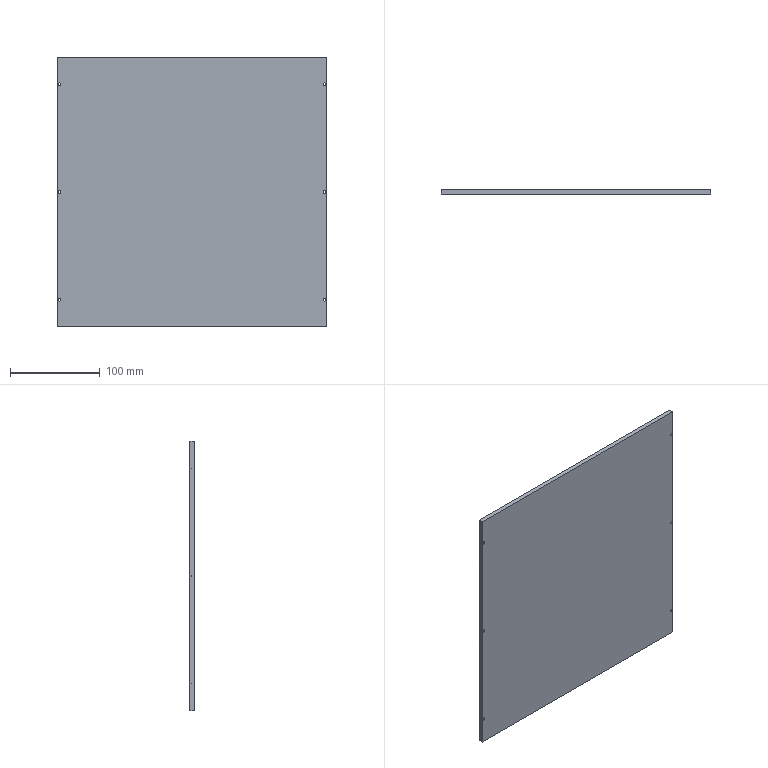Part | SolidWorks | features Extrusion 1, HoleWzd 1 | 1 solid | 30 faces | box 300 x 5 x 300 mm | volume 449761 mm3 | cylinder 12 | cone 12 | plane 6 | commonest cylinder face diameters 2.7 x12
STEP:
#1=CARTESIAN_POINT('',(147.5,0.,-118.65));
#2=VERTEX_POINT('',#1);
#3=CARTESIAN_POINT('',(147.5,0.,-121.35));
#4=VERTEX_POINT('',#3);
#5=CARTESIAN_POINT('',(147.5,0.,-120.));
#6=DIRECTION('',(0.,-1.,0.));
#7=DIRECTION('',(0.,0.,-1.));
#8=AXIS2_PLACEMENT_3D('',#5,#6,#7);
#9=CIRCLE('',#8,1.35);
#10=EDGE_CURVE('',#2,#4,#9,.T.);
#11=ORIENTED_EDGE('',*,*,#10,.T.);
#12=CARTESIAN_POINT('',(147.5,3.6,-121.35));
#13=VERTEX_POINT('',#12);
#14=CARTESIAN_POINT('',(147.5,5.,-121.35));
#15=DIRECTION('',(0.,1.,0.));
#16=VECTOR('',#15,1000.);
#17=LINE('',#14,#16);
#18=EDGE_CURVE('',#4,#13,#17,.T.);
#19=ORIENTED_EDGE('',*,*,#18,.T.);
#20=CARTESIAN_POINT('',(147.5,3.6,-118.65));
#21=VERTEX_POINT('',#20);
#22=CARTESIAN_POINT('',(147.5,3.6,-120.));
#23=DIRECTION('',(0.,1.,0.));
#24=DIRECTION('',(0.,0.,1.));
#25=AXIS2_PLACEMENT_3D('',#22,#23,#24);
#26=CIRCLE('',#25,1.35);
#27=EDGE_CURVE('',#13,#21,#26,.T.);
#28=ORIENTED_EDGE('',*,*,#27,.T.);
#29=CARTESIAN_POINT('',(147.5,5.,-118.65));
#30=DIRECTION('',(0.,1.,0.));
#31=VECTOR('',#30,1000.);
#32=LINE('',#29,#31);
#33=EDGE_CURVE('',#2,#21,#32,.T.);
#34=ORIENTED_EDGE('',*,*,#33,.F.);
#35=EDGE_LOOP('',(#11,#19,#28,#34));
#36=FACE_OUTER_BOUND('',#35,.T.);
#37=CARTESIAN_POINT('',(147.5,5.,-120.));
#38=DIRECTION('',(0.,1.,0.));
#39=DIRECTION('',(0.,0.,1.));
#40=AXIS2_PLACEMENT_3D('',#37,#38,#39);
#41=CYLINDRICAL_SURFACE('',#40,1.35);
#42=ADVANCED_FACE('',(#36),#41,.F.);
#43=ORIENTED_EDGE('',*,*,#27,.F.);
#44=CARTESIAN_POINT('',(147.5,5.,-122.75));
#45=VERTEX_POINT('',#44);
#46=CARTESIAN_POINT('',(147.5,5.,-122.75));
#47=DIRECTION('',(0.,0.7071,-0.7071));
#48=VECTOR('',#47,1000.);
#49=LINE('',#46,#48);
#50=EDGE_CURVE('',#13,#45,#49,.T.);
#51=ORIENTED_EDGE('',*,*,#50,.T.);
#52=CARTESIAN_POINT('',(147.5,5.,-117.25));
#53=VERTEX_POINT('',#52);
#54=CARTESIAN_POINT('',(147.5,5.,-120.));
#55=DIRECTION('',(0.,1.,0.));
#56=DIRECTION('',(0.,0.,1.));
#57=AXIS2_PLACEMENT_3D('',#54,#55,#56);
#58=CIRCLE('',#57,2.75);
#59=EDGE_CURVE('',#45,#53,#58,.T.);
#60=ORIENTED_EDGE('',*,*,#59,.T.);
#61=CARTESIAN_POINT('',(147.5,5.,-117.25));
#62=DIRECTION('',(0.,0.7071,0.7071));
#63=VECTOR('',#62,1000.);
#64=LINE('',#61,#63);
#65=EDGE_CURVE('',#21,#53,#64,.T.);
#66=ORIENTED_EDGE('',*,*,#65,.F.);
#67=EDGE_LOOP('',(#43,#51,#60,#66));
#68=FACE_OUTER_BOUND('',#67,.T.);
#69=CARTESIAN_POINT('',(147.5,5.,-120.));
#70=DIRECTION('',(0.,1.,0.));
#71=DIRECTION('',(0.,0.,1.));
#72=AXIS2_PLACEMENT_3D('',#69,#70,#71);
#73=CONICAL_SURFACE('',#72,2.75,0.7854);
#74=ADVANCED_FACE('',(#68),#73,.F.);
#75=CARTESIAN_POINT('',(147.5,0.,1.35));
#76=VERTEX_POINT('',#75);
#77=CARTESIAN_POINT('',(147.5,0.,-1.35));
#78=VERTEX_POINT('',#77);
#79=CARTESIAN_POINT('',(147.5,0.,0.));
#80=DIRECTION('',(0.,-1.,0.));
#81=DIRECTION('',(0.,0.,-1.));
#82=AXIS2_PLACEMENT_3D('',#79,#80,#81);
#83=CIRCLE('',#82,1.35);
#84=EDGE_CURVE('',#76,#78,#83,.T.);
#85=ORIENTED_EDGE('',*,*,#84,.T.);
#86=CARTESIAN_POINT('',(147.5,3.6,-1.35));
#87=VERTEX_POINT('',#86);
#88=CARTESIAN_POINT('',(147.5,5.,-1.35));
#89=DIRECTION('',(0.,1.,0.));
#90=VECTOR('',#89,1000.);
#91=LINE('',#88,#90);
#92=EDGE_CURVE('',#78,#87,#91,.T.);
#93=ORIENTED_EDGE('',*,*,#92,.T.);
#94=CARTESIAN_POINT('',(147.5,3.6,1.35));
#95=VERTEX_POINT('',#94);
#96=CARTESIAN_POINT('',(147.5,3.6,0.));
#97=DIRECTION('',(0.,1.,0.));
#98=DIRECTION('',(0.,0.,1.));
#99=AXIS2_PLACEMENT_3D('',#96,#97,#98);
#100=CIRCLE('',#99,1.35);
#101=EDGE_CURVE('',#87,#95,#100,.T.);
#102=ORIENTED_EDGE('',*,*,#101,.T.);
#103=CARTESIAN_POINT('',(147.5,5.,1.35));
#104=DIRECTION('',(0.,1.,0.));
#105=VECTOR('',#104,1000.);
#106=LINE('',#103,#105);
#107=EDGE_CURVE('',#76,#95,#106,.T.);
#108=ORIENTED_EDGE('',*,*,#107,.F.);
#109=EDGE_LOOP('',(#85,#93,#102,#108));
#110=FACE_OUTER_BOUND('',#109,.T.);
#111=CARTESIAN_POINT('',(147.5,5.,0.));
#112=DIRECTION('',(0.,1.,0.));
#113=DIRECTION('',(0.,0.,1.));
#114=AXIS2_PLACEMENT_3D('',#111,#112,#113);
#115=CYLINDRICAL_SURFACE('',#114,1.35);
#116=ADVANCED_FACE('',(#110),#115,.F.);
#117=ORIENTED_EDGE('',*,*,#101,.F.);
#118=CARTESIAN_POINT('',(147.5,5.,-2.75));
#119=VERTEX_POINT('',#118);
#120=CARTESIAN_POINT('',(147.5,5.,-2.75));
#121=DIRECTION('',(0.,0.7071,-0.7071));
#122=VECTOR('',#121,1000.);
#123=LINE('',#120,#122);
#124=EDGE_CURVE('',#87,#119,#123,.T.);
#125=ORIENTED_EDGE('',*,*,#124,.T.);
#126=CARTESIAN_POINT('',(147.5,5.,2.75));
#127=VERTEX_POINT('',#126);
#128=CARTESIAN_POINT('',(147.5,5.,0.));
#129=DIRECTION('',(0.,1.,0.));
#130=DIRECTION('',(0.,0.,1.));
#131=AXIS2_PLACEMENT_3D('',#128,#129,#130);
#132=CIRCLE('',#131,2.75);
#133=EDGE_CURVE('',#119,#127,#132,.T.);
#134=ORIENTED_EDGE('',*,*,#133,.T.);
#135=CARTESIAN_POINT('',(147.5,5.,2.75));
#136=DIRECTION('',(0.,0.7071,0.7071));
#137=VECTOR('',#136,1000.);
#138=LINE('',#135,#137);
#139=EDGE_CURVE('',#95,#127,#138,.T.);
#140=ORIENTED_EDGE('',*,*,#139,.F.);
#141=EDGE_LOOP('',(#117,#125,#134,#140));
#142=FACE_OUTER_BOUND('',#141,.T.);
#143=CARTESIAN_POINT('',(147.5,5.,0.));
#144=DIRECTION('',(0.,1.,0.));
#145=DIRECTION('',(0.,0.,1.));
#146=AXIS2_PLACEMENT_3D('',#143,#144,#145);
#147=CONICAL_SURFACE('',#146,2.75,0.7854);
#148=ADVANCED_FACE('',(#142),#147,.F.);
#149=CARTESIAN_POINT('',(147.5,0.,121.35));
#150=VERTEX_POINT('',#149);
#151=CARTESIAN_POINT('',(147.5,0.,118.65));
#152=VERTEX_POINT('',#151);
#153=CARTESIAN_POINT('',(147.5,0.,120.));
#154=DIRECTION('',(0.,-1.,0.));
#155=DIRECTION('',(0.,0.,-1.));
#156=AXIS2_PLACEMENT_3D('',#153,#154,#155);
#157=CIRCLE('',#156,1.35);
#158=EDGE_CURVE('',#150,#152,#157,.T.);
#159=ORIENTED_EDGE('',*,*,#158,.T.);
#160=CARTESIAN_POINT('',(147.5,3.6,118.65));
#161=VERTEX_POINT('',#160);
#162=CARTESIAN_POINT('',(147.5,5.,118.65));
#163=DIRECTION('',(0.,1.,0.));
#164=VECTOR('',#163,1000.);
#165=LINE('',#162,#164);
#166=EDGE_CURVE('',#152,#161,#165,.T.);
#167=ORIENTED_EDGE('',*,*,#166,.T.);
#168=CARTESIAN_POINT('',(147.5,3.6,121.35));
#169=VERTEX_POINT('',#168);
#170=CARTESIAN_POINT('',(147.5,3.6,120.));
#171=DIRECTION('',(0.,1.,0.));
#172=DIRECTION('',(0.,0.,1.));
#173=AXIS2_PLACEMENT_3D('',#170,#171,#172);
#174=CIRCLE('',#173,1.35);
#175=EDGE_CURVE('',#161,#169,#174,.T.);
#176=ORIENTED_EDGE('',*,*,#175,.T.);
#177=CARTESIAN_POINT('',(147.5,5.,121.35));
#178=DIRECTION('',(0.,1.,0.));
#179=VECTOR('',#178,1000.);
#180=LINE('',#177,#179);
#181=EDGE_CURVE('',#150,#169,#180,.T.);
#182=ORIENTED_EDGE('',*,*,#181,.F.);
#183=EDGE_LOOP('',(#159,#167,#176,#182));
#184=FACE_OUTER_BOUND('',#183,.T.);
#185=CARTESIAN_POINT('',(147.5,5.,120.));
#186=DIRECTION('',(0.,1.,0.));
#187=DIRECTION('',(0.,0.,1.));
#188=AXIS2_PLACEMENT_3D('',#185,#186,#187);
#189=CYLINDRICAL_SURFACE('',#188,1.35);
#190=ADVANCED_FACE('',(#184),#189,.F.);
#191=ORIENTED_EDGE('',*,*,#175,.F.);
#192=CARTESIAN_POINT('',(147.5,5.,117.25));
#193=VERTEX_POINT('',#192);
#194=CARTESIAN_POINT('',(147.5,5.,117.25));
#195=DIRECTION('',(0.,0.7071,-0.7071));
#196=VECTOR('',#195,1000.);
#197=LINE('',#194,#196);
#198=EDGE_CURVE('',#161,#193,#197,.T.);
#199=ORIENTED_EDGE('',*,*,#198,.T.);
#200=CARTESIAN_POINT('',(147.5,5.,122.75));
#201=VERTEX_POINT('',#200);
#202=CARTESIAN_POINT('',(147.5,5.,120.));
#203=DIRECTION('',(0.,1.,0.));
#204=DIRECTION('',(0.,0.,1.));
#205=AXIS2_PLACEMENT_3D('',#202,#203,#204);
#206=CIRCLE('',#205,2.75);
#207=EDGE_CURVE('',#193,#201,#206,.T.);
#208=ORIENTED_EDGE('',*,*,#207,.T.);
#209=CARTESIAN_POINT('',(147.5,5.,122.75));
#210=DIRECTION('',(0.,0.7071,0.7071));
#211=VECTOR('',#210,1000.);
#212=LINE('',#209,#211);
#213=EDGE_CURVE('',#169,#201,#212,.T.);
#214=ORIENTED_EDGE('',*,*,#213,.F.);
#215=EDGE_LOOP('',(#191,#199,#208,#214));
#216=FACE_OUTER_BOUND('',#215,.T.);
#217=CARTESIAN_POINT('',(147.5,5.,120.));
#218=DIRECTION('',(0.,1.,0.));
#219=DIRECTION('',(0.,0.,1.));
#220=AXIS2_PLACEMENT_3D('',#217,#218,#219);
#221=CONICAL_SURFACE('',#220,2.75,0.7854);
#222=ADVANCED_FACE('',(#216),#221,.F.);
#223=CARTESIAN_POINT('',(-147.5,0.,-118.65));
#224=VERTEX_POINT('',#223);
#225=CARTESIAN_POINT('',(-147.5,0.,-121.35));
#226=VERTEX_POINT('',#225);
#227=CARTESIAN_POINT('',(-147.5,0.,-120.));
#228=DIRECTION('',(0.,-1.,0.));
#229=DIRECTION('',(0.,0.,-1.));
#230=AXIS2_PLACEMENT_3D('',#227,#228,#229);
#231=CIRCLE('',#230,1.35);
#232=EDGE_CURVE('',#224,#226,#231,.T.);
#233=ORIENTED_EDGE('',*,*,#232,.T.);
#234=CARTESIAN_POINT('',(-147.5,3.6,-121.35));
#235=VERTEX_POINT('',#234);
#236=CARTESIAN_POINT('',(-147.5,5.,-121.35));
#237=DIRECTION('',(0.,1.,0.));
#238=VECTOR('',#237,1000.);
#239=LINE('',#236,#238);
#240=EDGE_CURVE('',#226,#235,#239,.T.);
#241=ORIENTED_EDGE('',*,*,#240,.T.);
#242=CARTESIAN_POINT('',(-147.5,3.6,-118.65));
#243=VERTEX_POINT('',#242);
#244=CARTESIAN_POINT('',(-147.5,3.6,-120.));
#245=DIRECTION('',(0.,1.,0.));
#246=DIRECTION('',(0.,0.,1.));
#247=AXIS2_PLACEMENT_3D('',#244,#245,#246);
#248=CIRCLE('',#247,1.35);
#249=EDGE_CURVE('',#235,#243,#248,.T.);
#250=ORIENTED_EDGE('',*,*,#249,.T.);
#251=CARTESIAN_POINT('',(-147.5,5.,-118.65));
#252=DIRECTION('',(0.,1.,0.));
#253=VECTOR('',#252,1000.);
#254=LINE('',#251,#253);
#255=EDGE_CURVE('',#224,#243,#254,.T.);
#256=ORIENTED_EDGE('',*,*,#255,.F.);
#257=EDGE_LOOP('',(#233,#241,#250,#256));
#258=FACE_OUTER_BOUND('',#257,.T.);
#259=CARTESIAN_POINT('',(-147.5,5.,-120.));
#260=DIRECTION('',(0.,1.,0.));
#261=DIRECTION('',(0.,0.,1.));
#262=AXIS2_PLACEMENT_3D('',#259,#260,#261);
#263=CYLINDRICAL_SURFACE('',#262,1.35);
#264=ADVANCED_FACE('',(#258),#263,.F.);
#265=ORIENTED_EDGE('',*,*,#249,.F.);
#266=CARTESIAN_POINT('',(-147.5,5.,-122.75));
#267=VERTEX_POINT('',#266);
#268=CARTESIAN_POINT('',(-147.5,5.,-122.75));
#269=DIRECTION('',(0.,0.7071,-0.7071));
#270=VECTOR('',#269,1000.);
#271=LINE('',#268,#270);
#272=EDGE_CURVE('',#235,#267,#271,.T.);
#273=ORIENTED_EDGE('',*,*,#272,.T.);
#274=CARTESIAN_POINT('',(-150.,5.,-121.146));
#275=VERTEX_POINT('',#274);
#276=CARTESIAN_POINT('',(-147.5,5.,-120.));
#277=DIRECTION('',(0.,1.,0.));
#278=DIRECTION('',(0.,0.,1.));
#279=AXIS2_PLACEMENT_3D('',#276,#277,#278);
#280=CIRCLE('',#279,2.75);
#281=EDGE_CURVE('',#267,#275,#280,.T.);
#282=ORIENTED_EDGE('',*,*,#281,.T.);
#283=CARTESIAN_POINT('',(-150.,5.,-118.854));
#284=VERTEX_POINT('',#283);
#285=CARTESIAN_POINT('',(-150.,5.,-118.854));
#286=CARTESIAN_POINT('',(-150.,4.924,-119.036));
#287=CARTESIAN_POINT('',(-150.,4.861,-119.225));
#288=CARTESIAN_POINT('',(-150.,4.774,-119.607));
#289=CARTESIAN_POINT('',(-150.,4.75,-119.802));
#290=CARTESIAN_POINT('',(-150.,4.75,-120.199));
#291=CARTESIAN_POINT('',(-150.,4.774,-120.394));
#292=CARTESIAN_POINT('',(-150.,4.861,-120.775));
#293=CARTESIAN_POINT('',(-150.,4.925,-120.965));
#294=CARTESIAN_POINT('',(-150.,5.,-121.146));
#295=B_SPLINE_CURVE_WITH_KNOTS('',3,(#285,#286,#287,#288,#289,#290,#291,#292,#293,#294),.UNSPECIFIED.,.F.,.F.,(4,2,2,2,4),(0.0116,0.01218,0.01277,0.01335,0.01394),.UNSPECIFIED.);
#296=EDGE_CURVE('',#284,#275,#295,.T.);
#297=ORIENTED_EDGE('',*,*,#296,.F.);
#298=CARTESIAN_POINT('',(-147.5,5.,-117.25));
#299=VERTEX_POINT('',#298);
#300=CARTESIAN_POINT('',(-147.5,5.,-120.));
#301=DIRECTION('',(0.,1.,0.));
#302=DIRECTION('',(0.,0.,1.));
#303=AXIS2_PLACEMENT_3D('',#300,#301,#302);
#304=CIRCLE('',#303,2.75);
#305=EDGE_CURVE('',#284,#299,#304,.T.);
#306=ORIENTED_EDGE('',*,*,#305,.T.);
#307=CARTESIAN_POINT('',(-147.5,5.,-117.25));
#308=DIRECTION('',(0.,0.7071,0.7071));
#309=VECTOR('',#308,1000.);
#310=LINE('',#307,#309);
#311=EDGE_CURVE('',#243,#299,#310,.T.);
#312=ORIENTED_EDGE('',*,*,#311,.F.);
#313=EDGE_LOOP('',(#265,#273,#282,#297,#306,#312));
#314=FACE_OUTER_BOUND('',#313,.T.);
#315=CARTESIAN_POINT('',(-147.5,5.,-120.));
#316=DIRECTION('',(0.,1.,0.));
#317=DIRECTION('',(0.,0.,1.));
#318=AXIS2_PLACEMENT_3D('',#315,#316,#317);
#319=CONICAL_SURFACE('',#318,2.75,0.7854);
#320=ADVANCED_FACE('',(#314),#319,.F.);
#321=CARTESIAN_POINT('',(-147.5,0.,1.35));
#322=VERTEX_POINT('',#321);
#323=CARTESIAN_POINT('',(-147.5,0.,-1.35));
#324=VERTEX_POINT('',#323);
#325=CARTESIAN_POINT('',(-147.5,0.,0.));
#326=DIRECTION('',(0.,-1.,0.));
#327=DIRECTION('',(0.,0.,-1.));
#328=AXIS2_PLACEMENT_3D('',#325,#326,#327);
#329=CIRCLE('',#328,1.35);
#330=EDGE_CURVE('',#322,#324,#329,.T.);
#331=ORIENTED_EDGE('',*,*,#330,.T.);
#332=CARTESIAN_POINT('',(-147.5,3.6,-1.35));
#333=VERTEX_POINT('',#332);
#334=CARTESIAN_POINT('',(-147.5,5.,-1.35));
#335=DIRECTION('',(0.,1.,0.));
#336=VECTOR('',#335,1000.);
#337=LINE('',#334,#336);
#338=EDGE_CURVE('',#324,#333,#337,.T.);
#339=ORIENTED_EDGE('',*,*,#338,.T.);
#340=CARTESIAN_POINT('',(-147.5,3.6,1.35));
#341=VERTEX_POINT('',#340);
#342=CARTESIAN_POINT('',(-147.5,3.6,0.));
#343=DIRECTION('',(0.,1.,0.));
#344=DIRECTION('',(0.,0.,1.));
#345=AXIS2_PLACEMENT_3D('',#342,#343,#344);
#346=CIRCLE('',#345,1.35);
#347=EDGE_CURVE('',#333,#341,#346,.T.);
#348=ORIENTED_EDGE('',*,*,#347,.T.);
#349=CARTESIAN_POINT('',(-147.5,5.,1.35));
#350=DIRECTION('',(0.,1.,0.));
#351=VECTOR('',#350,1000.);
#352=LINE('',#349,#351);
#353=EDGE_CURVE('',#322,#341,#352,.T.);
#354=ORIENTED_EDGE('',*,*,#353,.F.);
#355=EDGE_LOOP('',(#331,#339,#348,#354));
#356=FACE_OUTER_BOUND('',#355,.T.);
#357=CARTESIAN_POINT('',(-147.5,5.,0.));
#358=DIRECTION('',(0.,1.,0.));
#359=DIRECTION('',(0.,0.,1.));
#360=AXIS2_PLACEMENT_3D('',#357,#358,#359);
#361=CYLINDRICAL_SURFACE('',#360,1.35);
#362=ADVANCED_FACE('',(#356),#361,.F.);
#363=ORIENTED_EDGE('',*,*,#347,.F.);
#364=CARTESIAN_POINT('',(-147.5,5.,-2.75));
#365=VERTEX_POINT('',#364);
#366=CARTESIAN_POINT('',(-147.5,5.,-2.75));
#367=DIRECTION('',(0.,0.7071,-0.7071));
#368=VECTOR('',#367,1000.);
#369=LINE('',#366,#368);
#370=EDGE_CURVE('',#333,#365,#369,.T.);
#371=ORIENTED_EDGE('',*,*,#370,.T.);
#372=CARTESIAN_POINT('',(-150.,5.,-1.146));
#373=VERTEX_POINT('',#372);
#374=CARTESIAN_POINT('',(-147.5,5.,0.));
#375=DIRECTION('',(0.,1.,0.));
#376=DIRECTION('',(0.,0.,1.));
#377=AXIS2_PLACEMENT_3D('',#374,#375,#376);
#378=CIRCLE('',#377,2.75);
#379=EDGE_CURVE('',#365,#373,#378,.T.);
#380=ORIENTED_EDGE('',*,*,#379,.T.);
#381=CARTESIAN_POINT('',(-150.,5.,1.146));
#382=VERTEX_POINT('',#381);
#383=CARTESIAN_POINT('',(-150.,5.,1.146));
#384=CARTESIAN_POINT('',(-150.,4.924,0.9642));
#385=CARTESIAN_POINT('',(-150.,4.861,0.7753));
#386=CARTESIAN_POINT('',(-150.,4.774,0.3932));
#387=CARTESIAN_POINT('',(-150.,4.75,0.1976));
#388=CARTESIAN_POINT('',(-150.,4.75,-0.1993));
#389=CARTESIAN_POINT('',(-150.,4.774,-0.3936));
#390=CARTESIAN_POINT('',(-150.,4.861,-0.7755));
#391=CARTESIAN_POINT('',(-150.,4.925,-0.9646));
#392=CARTESIAN_POINT('',(-150.,5.,-1.146));
#393=B_SPLINE_CURVE_WITH_KNOTS('',3,(#383,#384,#385,#386,#387,#388,#389,#390,#391,#392),.UNSPECIFIED.,.F.,.F.,(4,2,2,2,4),(0.0116,0.01218,0.01277,0.01335,0.01394),.UNSPECIFIED.);
#394=EDGE_CURVE('',#382,#373,#393,.T.);
#395=ORIENTED_EDGE('',*,*,#394,.F.);
#396=CARTESIAN_POINT('',(-147.5,5.,2.75));
#397=VERTEX_POINT('',#396);
#398=CARTESIAN_POINT('',(-147.5,5.,0.));
#399=DIRECTION('',(0.,1.,0.));
#400=DIRECTION('',(0.,0.,1.));
#401=AXIS2_PLACEMENT_3D('',#398,#399,#400);
#402=CIRCLE('',#401,2.75);
#403=EDGE_CURVE('',#382,#397,#402,.T.);
#404=ORIENTED_EDGE('',*,*,#403,.T.);
#405=CARTESIAN_POINT('',(-147.5,5.,2.75));
#406=DIRECTION('',(0.,0.7071,0.7071));
#407=VECTOR('',#406,1000.);
#408=LINE('',#405,#407);
#409=EDGE_CURVE('',#341,#397,#408,.T.);
#410=ORIENTED_EDGE('',*,*,#409,.F.);
#411=EDGE_LOOP('',(#363,#371,#380,#395,#404,#410));
#412=FACE_OUTER_BOUND('',#411,.T.);
#413=CARTESIAN_POINT('',(-147.5,5.,0.));
#414=DIRECTION('',(0.,1.,0.));
#415=DIRECTION('',(0.,0.,1.));
#416=AXIS2_PLACEMENT_3D('',#413,#414,#415);
#417=CONICAL_SURFACE('',#416,2.75,0.7854);
#418=ADVANCED_FACE('',(#412),#417,.F.);
#419=CARTESIAN_POINT('',(-147.5,0.,121.35));
#420=VERTEX_POINT('',#419);
#421=CARTESIAN_POINT('',(-147.5,0.,118.65));
#422=VERTEX_POINT('',#421);
#423=CARTESIAN_POINT('',(-147.5,0.,120.));
#424=DIRECTION('',(0.,-1.,0.));
#425=DIRECTION('',(0.,0.,-1.));
#426=AXIS2_PLACEMENT_3D('',#423,#424,#425);
#427=CIRCLE('',#426,1.35);
#428=EDGE_CURVE('',#420,#422,#427,.T.);
#429=ORIENTED_EDGE('',*,*,#428,.T.);
#430=CARTESIAN_POINT('',(-147.5,3.6,118.65));
#431=VERTEX_POINT('',#430);
#432=CARTESIAN_POINT('',(-147.5,5.,118.65));
#433=DIRECTION('',(0.,1.,0.));
#434=VECTOR('',#433,1000.);
#435=LINE('',#432,#434);
#436=EDGE_CURVE('',#422,#431,#435,.T.);
#437=ORIENTED_EDGE('',*,*,#436,.T.);
#438=CARTESIAN_POINT('',(-147.5,3.6,121.35));
#439=VERTEX_POINT('',#438);
#440=CARTESIAN_POINT('',(-147.5,3.6,120.));
#441=DIRECTION('',(0.,1.,0.));
#442=DIRECTION('',(0.,0.,1.));
#443=AXIS2_PLACEMENT_3D('',#440,#441,#442);
#444=CIRCLE('',#443,1.35);
#445=EDGE_CURVE('',#431,#439,#444,.T.);
#446=ORIENTED_EDGE('',*,*,#445,.T.);
#447=CARTESIAN_POINT('',(-147.5,5.,121.35));
#448=DIRECTION('',(0.,1.,0.));
#449=VECTOR('',#448,1000.);
#450=LINE('',#447,#449);
#451=EDGE_CURVE('',#420,#439,#450,.T.);
#452=ORIENTED_EDGE('',*,*,#451,.F.);
#453=EDGE_LOOP('',(#429,#437,#446,#452));
#454=FACE_OUTER_BOUND('',#453,.T.);
#455=CARTESIAN_POINT('',(-147.5,5.,120.));
#456=DIRECTION('',(0.,1.,0.));
#457=DIRECTION('',(0.,0.,1.));
#458=AXIS2_PLACEMENT_3D('',#455,#456,#457);
#459=CYLINDRICAL_SURFACE('',#458,1.35);
#460=ADVANCED_FACE('',(#454),#459,.F.);
#461=ORIENTED_EDGE('',*,*,#445,.F.);
#462=CARTESIAN_POINT('',(-147.5,5.,117.25));
#463=VERTEX_POINT('',#462);
#464=CARTESIAN_POINT('',(-147.5,5.,117.25));
#465=DIRECTION('',(0.,0.7071,-0.7071));
#466=VECTOR('',#465,1000.);
#467=LINE('',#464,#466);
#468=EDGE_CURVE('',#431,#463,#467,.T.);
#469=ORIENTED_EDGE('',*,*,#468,.T.);
#470=CARTESIAN_POINT('',(-150.,5.,118.854));
#471=VERTEX_POINT('',#470);
#472=CARTESIAN_POINT('',(-147.5,5.,120.));
#473=DIRECTION('',(0.,1.,0.));
#474=DIRECTION('',(0.,0.,1.));
#475=AXIS2_PLACEMENT_3D('',#472,#473,#474);
#476=CIRCLE('',#475,2.75);
#477=EDGE_CURVE('',#463,#471,#476,.T.);
#478=ORIENTED_EDGE('',*,*,#477,.T.);
#479=CARTESIAN_POINT('',(-150.,5.,121.146));
#480=VERTEX_POINT('',#479);
#481=CARTESIAN_POINT('',(-150.,5.,121.146));
#482=CARTESIAN_POINT('',(-150.,4.924,120.964));
#483=CARTESIAN_POINT('',(-150.,4.861,120.775));
#484=CARTESIAN_POINT('',(-150.,4.774,120.393));
#485=CARTESIAN_POINT('',(-150.,4.75,120.198));
#486=CARTESIAN_POINT('',(-150.,4.75,119.801));
#487=CARTESIAN_POINT('',(-150.,4.774,119.606));
#488=CARTESIAN_POINT('',(-150.,4.861,119.225));
#489=CARTESIAN_POINT('',(-150.,4.925,119.035));
#490=CARTESIAN_POINT('',(-150.,5.,118.854));
#491=B_SPLINE_CURVE_WITH_KNOTS('',3,(#481,#482,#483,#484,#485,#486,#487,#488,#489,#490),.UNSPECIFIED.,.F.,.F.,(4,2,2,2,4),(0.0116,0.01218,0.01277,0.01335,0.01394),.UNSPECIFIED.);
#492=EDGE_CURVE('',#480,#471,#491,.T.);
#493=ORIENTED_EDGE('',*,*,#492,.F.);
#494=CARTESIAN_POINT('',(-147.5,5.,122.75));
#495=VERTEX_POINT('',#494);
#496=CARTESIAN_POINT('',(-147.5,5.,120.));
#497=DIRECTION('',(0.,1.,0.));
#498=DIRECTION('',(0.,0.,1.));
#499=AXIS2_PLACEMENT_3D('',#496,#497,#498);
#500=CIRCLE('',#499,2.75);
#501=EDGE_CURVE('',#480,#495,#500,.T.);
#502=ORIENTED_EDGE('',*,*,#501,.T.);
#503=CARTESIAN_POINT('',(-147.5,5.,122.75));
#504=DIRECTION('',(0.,0.7071,0.7071));
#505=VECTOR('',#504,1000.);
#506=LINE('',#503,#505);
#507=EDGE_CURVE('',#439,#495,#506,.T.);
#508=ORIENTED_EDGE('',*,*,#507,.F.);
#509=EDGE_LOOP('',(#461,#469,#478,#493,#502,#508));
#510=FACE_OUTER_BOUND('',#509,.T.);
#511=CARTESIAN_POINT('',(-147.5,5.,120.));
#512=DIRECTION('',(0.,1.,0.));
#513=DIRECTION('',(0.,0.,1.));
#514=AXIS2_PLACEMENT_3D('',#511,#512,#513);
#515=CONICAL_SURFACE('',#514,2.75,0.7854);
#516=ADVANCED_FACE('',(#510),#515,.F.);
#517=CARTESIAN_POINT('',(150.,5.,-1.146));
#518=VERTEX_POINT('',#517);
#519=CARTESIAN_POINT('',(150.,5.,-118.854));
#520=VERTEX_POINT('',#519);
#521=CARTESIAN_POINT('',(150.,5.,150.));
#522=DIRECTION('',(0.,0.,-1.));
#523=VECTOR('',#522,1000.);
#524=LINE('',#521,#523);
#525=EDGE_CURVE('',#518,#520,#524,.T.);
#526=ORIENTED_EDGE('',*,*,#525,.T.);
#527=CARTESIAN_POINT('',(147.5,5.,-120.));
#528=DIRECTION('',(0.,1.,0.));
#529=DIRECTION('',(0.,0.,1.));
#530=AXIS2_PLACEMENT_3D('',#527,#528,#529);
#531=CIRCLE('',#530,2.75);
#532=EDGE_CURVE('',#53,#520,#531,.T.);
#533=ORIENTED_EDGE('',*,*,#532,.F.);
#534=ORIENTED_EDGE('',*,*,#59,.F.);
#535=CARTESIAN_POINT('',(150.,5.,-121.146));
#536=VERTEX_POINT('',#535);
#537=CARTESIAN_POINT('',(147.5,5.,-120.));
#538=DIRECTION('',(0.,1.,0.));
#539=DIRECTION('',(0.,0.,1.));
#540=AXIS2_PLACEMENT_3D('',#537,#538,#539);
#541=CIRCLE('',#540,2.75);
#542=EDGE_CURVE('',#536,#45,#541,.T.);
#543=ORIENTED_EDGE('',*,*,#542,.F.);
#544=CARTESIAN_POINT('',(150.,5.,-150.));
#545=VERTEX_POINT('',#544);
#546=CARTESIAN_POINT('',(150.,5.,150.));
#547=DIRECTION('',(0.,0.,-1.));
#548=VECTOR('',#547,1000.);
#549=LINE('',#546,#548);
#550=EDGE_CURVE('',#536,#545,#549,.T.);
#551=ORIENTED_EDGE('',*,*,#550,.T.);
#552=CARTESIAN_POINT('',(-150.,5.,-150.));
#553=VERTEX_POINT('',#552);
#554=CARTESIAN_POINT('',(-150.,5.,-150.));
#555=DIRECTION('',(-1.,0.,0.));
#556=VECTOR('',#555,1000.);
#557=LINE('',#554,#556);
#558=EDGE_CURVE('',#545,#553,#557,.T.);
#559=ORIENTED_EDGE('',*,*,#558,.T.);
#560=CARTESIAN_POINT('',(-150.,5.,150.));
#561=DIRECTION('',(0.,0.,1.));
#562=VECTOR('',#561,1000.);
#563=LINE('',#560,#562);
#564=EDGE_CURVE('',#553,#275,#563,.T.);
#565=ORIENTED_EDGE('',*,*,#564,.T.);
#566=ORIENTED_EDGE('',*,*,#281,.F.);
#567=CARTESIAN_POINT('',(-147.5,5.,-120.));
#568=DIRECTION('',(0.,1.,0.));
#569=DIRECTION('',(0.,0.,1.));
#570=AXIS2_PLACEMENT_3D('',#567,#568,#569);
#571=CIRCLE('',#570,2.75);
#572=EDGE_CURVE('',#299,#267,#571,.T.);
#573=ORIENTED_EDGE('',*,*,#572,.F.);
#574=ORIENTED_EDGE('',*,*,#305,.F.);
#575=CARTESIAN_POINT('',(-150.,5.,150.));
#576=DIRECTION('',(0.,0.,1.));
#577=VECTOR('',#576,1000.);
#578=LINE('',#575,#577);
#579=EDGE_CURVE('',#284,#373,#578,.T.);
#580=ORIENTED_EDGE('',*,*,#579,.T.);
#581=ORIENTED_EDGE('',*,*,#379,.F.);
#582=CARTESIAN_POINT('',(-147.5,5.,0.));
#583=DIRECTION('',(0.,1.,0.));
#584=DIRECTION('',(0.,0.,1.));
#585=AXIS2_PLACEMENT_3D('',#582,#583,#584);
#586=CIRCLE('',#585,2.75);
#587=EDGE_CURVE('',#397,#365,#586,.T.);
#588=ORIENTED_EDGE('',*,*,#587,.F.);
#589=ORIENTED_EDGE('',*,*,#403,.F.);
#590=CARTESIAN_POINT('',(-150.,5.,150.));
#591=DIRECTION('',(0.,0.,1.));
#592=VECTOR('',#591,1000.);
#593=LINE('',#590,#592);
#594=EDGE_CURVE('',#382,#471,#593,.T.);
#595=ORIENTED_EDGE('',*,*,#594,.T.);
#596=ORIENTED_EDGE('',*,*,#477,.F.);
#597=CARTESIAN_POINT('',(-147.5,5.,120.));
#598=DIRECTION('',(0.,1.,0.));
#599=DIRECTION('',(0.,0.,1.));
#600=AXIS2_PLACEMENT_3D('',#597,#598,#599);
#601=CIRCLE('',#600,2.75);
#602=EDGE_CURVE('',#495,#463,#601,.T.);
#603=ORIENTED_EDGE('',*,*,#602,.F.);
#604=ORIENTED_EDGE('',*,*,#501,.F.);
#605=CARTESIAN_POINT('',(-150.,5.,150.));
#606=VERTEX_POINT('',#605);
#607=CARTESIAN_POINT('',(-150.,5.,150.));
#608=DIRECTION('',(0.,0.,1.));
#609=VECTOR('',#608,1000.);
#610=LINE('',#607,#609);
#611=EDGE_CURVE('',#480,#606,#610,.T.);
#612=ORIENTED_EDGE('',*,*,#611,.T.);
#613=CARTESIAN_POINT('',(150.,5.,150.));
#614=VERTEX_POINT('',#613);
#615=CARTESIAN_POINT('',(-150.,5.,150.));
#616=DIRECTION('',(1.,0.,0.));
#617=VECTOR('',#616,1000.);
#618=LINE('',#615,#617);
#619=EDGE_CURVE('',#606,#614,#618,.T.);
#620=ORIENTED_EDGE('',*,*,#619,.T.);
#621=CARTESIAN_POINT('',(150.,5.,121.146));
#622=VERTEX_POINT('',#621);
#623=CARTESIAN_POINT('',(150.,5.,150.));
#624=DIRECTION('',(0.,0.,-1.));
#625=VECTOR('',#624,1000.);
#626=LINE('',#623,#625);
#627=EDGE_CURVE('',#614,#622,#626,.T.);
#628=ORIENTED_EDGE('',*,*,#627,.T.);
#629=CARTESIAN_POINT('',(147.5,5.,120.));
#630=DIRECTION('',(0.,1.,0.));
#631=DIRECTION('',(0.,0.,1.));
#632=AXIS2_PLACEMENT_3D('',#629,#630,#631);
#633=CIRCLE('',#632,2.75);
#634=EDGE_CURVE('',#201,#622,#633,.T.);
#635=ORIENTED_EDGE('',*,*,#634,.F.);
#636=ORIENTED_EDGE('',*,*,#207,.F.);
#637=CARTESIAN_POINT('',(150.,5.,118.854));
#638=VERTEX_POINT('',#637);
#639=CARTESIAN_POINT('',(147.5,5.,120.));
#640=DIRECTION('',(0.,1.,0.));
#641=DIRECTION('',(0.,0.,1.));
#642=AXIS2_PLACEMENT_3D('',#639,#640,#641);
#643=CIRCLE('',#642,2.75);
#644=EDGE_CURVE('',#638,#193,#643,.T.);
#645=ORIENTED_EDGE('',*,*,#644,.F.);
#646=CARTESIAN_POINT('',(150.,5.,1.146));
#647=VERTEX_POINT('',#646);
#648=CARTESIAN_POINT('',(150.,5.,150.));
#649=DIRECTION('',(0.,0.,-1.));
#650=VECTOR('',#649,1000.);
#651=LINE('',#648,#650);
#652=EDGE_CURVE('',#638,#647,#651,.T.);
#653=ORIENTED_EDGE('',*,*,#652,.T.);
#654=CARTESIAN_POINT('',(147.5,5.,0.));
#655=DIRECTION('',(0.,1.,0.));
#656=DIRECTION('',(0.,0.,1.));
#657=AXIS2_PLACEMENT_3D('',#654,#655,#656);
#658=CIRCLE('',#657,2.75);
#659=EDGE_CURVE('',#127,#647,#658,.T.);
#660=ORIENTED_EDGE('',*,*,#659,.F.);
#661=ORIENTED_EDGE('',*,*,#133,.F.);
#662=CARTESIAN_POINT('',(147.5,5.,0.));
#663=DIRECTION('',(0.,1.,0.));
#664=DIRECTION('',(0.,0.,1.));
#665=AXIS2_PLACEMENT_3D('',#662,#663,#664);
#666=CIRCLE('',#665,2.75);
#667=EDGE_CURVE('',#518,#119,#666,.T.);
#668=ORIENTED_EDGE('',*,*,#667,.F.);
#669=EDGE_LOOP('',(#526,#533,#534,#543,#551,#559,#565,#566,#573,#574,#580,#581,#588,#589,#595,#596,#603,#604,#612,#620,#628,#635,#636,#645,#653,#660,#661,#668));
#670=FACE_OUTER_BOUND('',#669,.T.);
#671=CARTESIAN_POINT('',(0.,5.,0.));
#672=DIRECTION('',(0.,-1.,0.));
#673=DIRECTION('',(0.,0.,-1.));
#674=AXIS2_PLACEMENT_3D('',#671,#672,#673);
#675=PLANE('',#674);
#676=ADVANCED_FACE('',(#670),#675,.F.);
#677=ORIENTED_EDGE('',*,*,#550,.F.);
#678=CARTESIAN_POINT('',(150.,5.,-121.146));
#679=CARTESIAN_POINT('',(150.,4.925,-120.965));
#680=CARTESIAN_POINT('',(150.,4.861,-120.775));
#681=CARTESIAN_POINT('',(150.,4.774,-120.394));
#682=CARTESIAN_POINT('',(150.,4.75,-120.199));
#683=CARTESIAN_POINT('',(150.,4.75,-119.802));
#684=CARTESIAN_POINT('',(150.,4.774,-119.607));
#685=CARTESIAN_POINT('',(150.,4.861,-119.225));
#686=CARTESIAN_POINT('',(150.,4.924,-119.036));
#687=CARTESIAN_POINT('',(150.,5.,-118.854));
#688=B_SPLINE_CURVE_WITH_KNOTS('',3,(#678,#679,#680,#681,#682,#683,#684,#685,#686,#687),.UNSPECIFIED.,.F.,.F.,(4,2,2,2,4),(0.01086,0.01144,0.01203,0.01261,0.01319),.UNSPECIFIED.);
#689=EDGE_CURVE('',#536,#520,#688,.T.);
#690=ORIENTED_EDGE('',*,*,#689,.T.);
#691=ORIENTED_EDGE('',*,*,#525,.F.);
#692=CARTESIAN_POINT('',(150.,5.,-1.146));
#693=CARTESIAN_POINT('',(150.,4.925,-0.9646));
#694=CARTESIAN_POINT('',(150.,4.861,-0.7755));
#695=CARTESIAN_POINT('',(150.,4.774,-0.3936));
#696=CARTESIAN_POINT('',(150.,4.75,-0.1993));
#697=CARTESIAN_POINT('',(150.,4.75,0.1976));
#698=CARTESIAN_POINT('',(150.,4.774,0.3932));
#699=CARTESIAN_POINT('',(150.,4.861,0.7753));
#700=CARTESIAN_POINT('',(150.,4.924,0.9642));
#701=CARTESIAN_POINT('',(150.,5.,1.146));
#702=B_SPLINE_CURVE_WITH_KNOTS('',3,(#692,#693,#694,#695,#696,#697,#698,#699,#700,#701),.UNSPECIFIED.,.F.,.F.,(4,2,2,2,4),(0.01086,0.01144,0.01203,0.01261,0.01319),.UNSPECIFIED.);
#703=EDGE_CURVE('',#518,#647,#702,.T.);
#704=ORIENTED_EDGE('',*,*,#703,.T.);
#705=ORIENTED_EDGE('',*,*,#652,.F.);
#706=CARTESIAN_POINT('',(150.,5.,118.854));
#707=CARTESIAN_POINT('',(150.,4.925,119.035));
#708=CARTESIAN_POINT('',(150.,4.861,119.225));
#709=CARTESIAN_POINT('',(150.,4.774,119.606));
#710=CARTESIAN_POINT('',(150.,4.75,119.801));
#711=CARTESIAN_POINT('',(150.,4.75,120.198));
#712=CARTESIAN_POINT('',(150.,4.774,120.393));
#713=CARTESIAN_POINT('',(150.,4.861,120.775));
#714=CARTESIAN_POINT('',(150.,4.924,120.964));
#715=CARTESIAN_POINT('',(150.,5.,121.146));
#716=B_SPLINE_CURVE_WITH_KNOTS('',3,(#706,#707,#708,#709,#710,#711,#712,#713,#714,#715),.UNSPECIFIED.,.F.,.F.,(4,2,2,2,4),(0.01086,0.01144,0.01203,0.01261,0.01319),.UNSPECIFIED.);
#717=EDGE_CURVE('',#638,#622,#716,.T.);
#718=ORIENTED_EDGE('',*,*,#717,.T.);
#719=ORIENTED_EDGE('',*,*,#627,.F.);
#720=CARTESIAN_POINT('',(150.,0.,150.));
#721=VERTEX_POINT('',#720);
#722=CARTESIAN_POINT('',(150.,5.,150.));
#723=DIRECTION('',(0.,-1.,0.));
#724=VECTOR('',#723,1000.);
#725=LINE('',#722,#724);
#726=EDGE_CURVE('',#614,#721,#725,.T.);
#727=ORIENTED_EDGE('',*,*,#726,.T.);
#728=CARTESIAN_POINT('',(150.,0.,-150.));
#729=VERTEX_POINT('',#728);
#730=CARTESIAN_POINT('',(150.,0.,150.));
#731=DIRECTION('',(0.,0.,-1.));
#732=VECTOR('',#731,1000.);
#733=LINE('',#730,#732);
#734=EDGE_CURVE('',#721,#729,#733,.T.);
#735=ORIENTED_EDGE('',*,*,#734,.T.);
#736=CARTESIAN_POINT('',(150.,5.,-150.));
#737=DIRECTION('',(0.,-1.,0.));
#738=VECTOR('',#737,1000.);
#739=LINE('',#736,#738);
#740=EDGE_CURVE('',#545,#729,#739,.T.);
#741=ORIENTED_EDGE('',*,*,#740,.F.);
#742=EDGE_LOOP('',(#677,#690,#691,#704,#705,#718,#719,#727,#735,#741));
#743=FACE_OUTER_BOUND('',#742,.T.);
#744=CARTESIAN_POINT('',(150.,5.,150.));
#745=DIRECTION('',(-1.,0.,0.));
#746=DIRECTION('',(0.,0.,1.));
#747=AXIS2_PLACEMENT_3D('',#744,#745,#746);
#748=PLANE('',#747);
#749=ADVANCED_FACE('',(#743),#748,.F.);
#750=CARTESIAN_POINT('',(-150.,0.,-150.));
#751=VERTEX_POINT('',#750);
#752=CARTESIAN_POINT('',(-150.,0.,-150.));
#753=DIRECTION('',(-1.,0.,0.));
#754=VECTOR('',#753,1000.);
#755=LINE('',#752,#754);
#756=EDGE_CURVE('',#729,#751,#755,.T.);
#757=ORIENTED_EDGE('',*,*,#756,.T.);
#758=CARTESIAN_POINT('',(-150.,5.,-150.));
#759=DIRECTION('',(0.,-1.,0.));
#760=VECTOR('',#759,1000.);
#761=LINE('',#758,#760);
#762=EDGE_CURVE('',#553,#751,#761,.T.);
#763=ORIENTED_EDGE('',*,*,#762,.F.);
#764=ORIENTED_EDGE('',*,*,#558,.F.);
#765=ORIENTED_EDGE('',*,*,#740,.T.);
#766=EDGE_LOOP('',(#757,#763,#764,#765));
#767=FACE_OUTER_BOUND('',#766,.T.);
#768=CARTESIAN_POINT('',(-150.,5.,-150.));
#769=DIRECTION('',(0.,0.,1.));
#770=DIRECTION('',(1.,0.,0.));
#771=AXIS2_PLACEMENT_3D('',#768,#769,#770);
#772=PLANE('',#771);
#773=ADVANCED_FACE('',(#767),#772,.F.);
#774=ORIENTED_EDGE('',*,*,#579,.F.);
#775=ORIENTED_EDGE('',*,*,#296,.T.);
#776=ORIENTED_EDGE('',*,*,#564,.F.);
#777=ORIENTED_EDGE('',*,*,#762,.T.);
#778=CARTESIAN_POINT('',(-150.,0.,150.));
#779=VERTEX_POINT('',#778);
#780=CARTESIAN_POINT('',(-150.,0.,150.));
#781=DIRECTION('',(0.,0.,1.));
#782=VECTOR('',#781,1000.);
#783=LINE('',#780,#782);
#784=EDGE_CURVE('',#751,#779,#783,.T.);
#785=ORIENTED_EDGE('',*,*,#784,.T.);
#786=CARTESIAN_POINT('',(-150.,5.,150.));
#787=DIRECTION('',(0.,-1.,0.));
#788=VECTOR('',#787,1000.);
#789=LINE('',#786,#788);
#790=EDGE_CURVE('',#606,#779,#789,.T.);
#791=ORIENTED_EDGE('',*,*,#790,.F.);
#792=ORIENTED_EDGE('',*,*,#611,.F.);
#793=ORIENTED_EDGE('',*,*,#492,.T.);
#794=ORIENTED_EDGE('',*,*,#594,.F.);
#795=ORIENTED_EDGE('',*,*,#394,.T.);
#796=EDGE_LOOP('',(#774,#775,#776,#777,#785,#791,#792,#793,#794,#795));
#797=FACE_OUTER_BOUND('',#796,.T.);
#798=CARTESIAN_POINT('',(-150.,5.,150.));
#799=DIRECTION('',(1.,0.,0.));
#800=DIRECTION('',(0.,0.,-1.));
#801=AXIS2_PLACEMENT_3D('',#798,#799,#800);
#802=PLANE('',#801);
#803=ADVANCED_FACE('',(#797),#802,.F.);
#804=CARTESIAN_POINT('',(-150.,0.,150.));
#805=DIRECTION('',(1.,0.,0.));
#806=VECTOR('',#805,1000.);
#807=LINE('',#804,#806);
#808=EDGE_CURVE('',#779,#721,#807,.T.);
#809=ORIENTED_EDGE('',*,*,#808,.T.);
#810=ORIENTED_EDGE('',*,*,#726,.F.);
#811=ORIENTED_EDGE('',*,*,#619,.F.);
#812=ORIENTED_EDGE('',*,*,#790,.T.);
#813=EDGE_LOOP('',(#809,#810,#811,#812));
#814=FACE_OUTER_BOUND('',#813,.T.);
#815=CARTESIAN_POINT('',(-150.,5.,150.));
#816=DIRECTION('',(0.,0.,-1.));
#817=DIRECTION('',(-1.,0.,0.));
#818=AXIS2_PLACEMENT_3D('',#815,#816,#817);
#819=PLANE('',#818);
#820=ADVANCED_FACE('',(#814),#819,.F.);
#821=ORIENTED_EDGE('',*,*,#10,.F.);
#822=CARTESIAN_POINT('',(147.5,0.,-120.));
#823=DIRECTION('',(0.,-1.,0.));
#824=DIRECTION('',(0.,0.,-1.));
#825=AXIS2_PLACEMENT_3D('',#822,#823,#824);
#826=CIRCLE('',#825,1.35);
#827=EDGE_CURVE('',#4,#2,#826,.T.);
#828=ORIENTED_EDGE('',*,*,#827,.F.);
#829=EDGE_LOOP('',(#821,#828));
#830=FACE_BOUND('',#829,.T.);
#831=ORIENTED_EDGE('',*,*,#84,.F.);
#832=CARTESIAN_POINT('',(147.5,0.,0.));
#833=DIRECTION('',(0.,-1.,0.));
#834=DIRECTION('',(0.,0.,-1.));
#835=AXIS2_PLACEMENT_3D('',#832,#833,#834);
#836=CIRCLE('',#835,1.35);
#837=EDGE_CURVE('',#78,#76,#836,.T.);
#838=ORIENTED_EDGE('',*,*,#837,.F.);
#839=EDGE_LOOP('',(#831,#838));
#840=FACE_BOUND('',#839,.T.);
#841=ORIENTED_EDGE('',*,*,#158,.F.);
#842=CARTESIAN_POINT('',(147.5,0.,120.));
#843=DIRECTION('',(0.,-1.,0.));
#844=DIRECTION('',(0.,0.,-1.));
#845=AXIS2_PLACEMENT_3D('',#842,#843,#844);
#846=CIRCLE('',#845,1.35);
#847=EDGE_CURVE('',#152,#150,#846,.T.);
#848=ORIENTED_EDGE('',*,*,#847,.F.);
#849=EDGE_LOOP('',(#841,#848));
#850=FACE_BOUND('',#849,.T.);
#851=ORIENTED_EDGE('',*,*,#232,.F.);
#852=CARTESIAN_POINT('',(-147.5,0.,-120.));
#853=DIRECTION('',(0.,-1.,0.));
#854=DIRECTION('',(0.,0.,-1.));
#855=AXIS2_PLACEMENT_3D('',#852,#853,#854);
#856=CIRCLE('',#855,1.35);
#857=EDGE_CURVE('',#226,#224,#856,.T.);
#858=ORIENTED_EDGE('',*,*,#857,.F.);
#859=EDGE_LOOP('',(#851,#858));
#860=FACE_BOUND('',#859,.T.);
#861=ORIENTED_EDGE('',*,*,#330,.F.);
#862=CARTESIAN_POINT('',(-147.5,0.,0.));
#863=DIRECTION('',(0.,-1.,0.));
#864=DIRECTION('',(0.,0.,-1.));
#865=AXIS2_PLACEMENT_3D('',#862,#863,#864);
#866=CIRCLE('',#865,1.35);
#867=EDGE_CURVE('',#324,#322,#866,.T.);
#868=ORIENTED_EDGE('',*,*,#867,.F.);
#869=EDGE_LOOP('',(#861,#868));
#870=FACE_BOUND('',#869,.T.);
#871=ORIENTED_EDGE('',*,*,#428,.F.);
#872=CARTESIAN_POINT('',(-147.5,0.,120.));
#873=DIRECTION('',(0.,-1.,0.));
#874=DIRECTION('',(0.,0.,-1.));
#875=AXIS2_PLACEMENT_3D('',#872,#873,#874);
#876=CIRCLE('',#875,1.35);
#877=EDGE_CURVE('',#422,#420,#876,.T.);
#878=ORIENTED_EDGE('',*,*,#877,.F.);
#879=EDGE_LOOP('',(#871,#878));
#880=FACE_BOUND('',#879,.T.);
#881=ORIENTED_EDGE('',*,*,#734,.F.);
#882=ORIENTED_EDGE('',*,*,#808,.F.);
#883=ORIENTED_EDGE('',*,*,#784,.F.);
#884=ORIENTED_EDGE('',*,*,#756,.F.);
#885=EDGE_LOOP('',(#881,#882,#883,#884));
#886=FACE_OUTER_BOUND('',#885,.T.);
#887=CARTESIAN_POINT('',(0.,0.,0.));
#888=DIRECTION('',(0.,-1.,0.));
#889=DIRECTION('',(0.,0.,-1.));
#890=AXIS2_PLACEMENT_3D('',#887,#888,#889);
#891=PLANE('',#890);
#892=ADVANCED_FACE('',(#830,#840,#850,#860,#870,#880,#886),#891,.T.);
#893=ORIENTED_EDGE('',*,*,#468,.F.);
#894=CARTESIAN_POINT('',(-147.5,3.6,120.));
#895=DIRECTION('',(0.,1.,0.));
#896=DIRECTION('',(0.,0.,1.));
#897=AXIS2_PLACEMENT_3D('',#894,#895,#896);
#898=CIRCLE('',#897,1.35);
#899=EDGE_CURVE('',#439,#431,#898,.T.);
#900=ORIENTED_EDGE('',*,*,#899,.F.);
#901=ORIENTED_EDGE('',*,*,#507,.T.);
#902=ORIENTED_EDGE('',*,*,#602,.T.);
#903=EDGE_LOOP('',(#893,#900,#901,#902));
#904=FACE_OUTER_BOUND('',#903,.T.);
#905=CARTESIAN_POINT('',(-147.5,5.,120.));
#906=DIRECTION('',(0.,1.,0.));
#907=DIRECTION('',(0.,0.,1.));
#908=AXIS2_PLACEMENT_3D('',#905,#906,#907);
#909=CONICAL_SURFACE('',#908,2.75,0.7854);
#910=ADVANCED_FACE('',(#904),#909,.F.);
#911=ORIENTED_EDGE('',*,*,#436,.F.);
#912=ORIENTED_EDGE('',*,*,#877,.T.);
#913=ORIENTED_EDGE('',*,*,#451,.T.);
#914=ORIENTED_EDGE('',*,*,#899,.T.);
#915=EDGE_LOOP('',(#911,#912,#913,#914));
#916=FACE_OUTER_BOUND('',#915,.T.);
#917=CARTESIAN_POINT('',(-147.5,5.,120.));
#918=DIRECTION('',(0.,1.,0.));
#919=DIRECTION('',(0.,0.,1.));
#920=AXIS2_PLACEMENT_3D('',#917,#918,#919);
#921=CYLINDRICAL_SURFACE('',#920,1.35);
#922=ADVANCED_FACE('',(#916),#921,.F.);
#923=ORIENTED_EDGE('',*,*,#370,.F.);
#924=CARTESIAN_POINT('',(-147.5,3.6,0.));
#925=DIRECTION('',(0.,1.,0.));
#926=DIRECTION('',(0.,0.,1.));
#927=AXIS2_PLACEMENT_3D('',#924,#925,#926);
#928=CIRCLE('',#927,1.35);
#929=EDGE_CURVE('',#341,#333,#928,.T.);
#930=ORIENTED_EDGE('',*,*,#929,.F.);
#931=ORIENTED_EDGE('',*,*,#409,.T.);
#932=ORIENTED_EDGE('',*,*,#587,.T.);
#933=EDGE_LOOP('',(#923,#930,#931,#932));
#934=FACE_OUTER_BOUND('',#933,.T.);
#935=CARTESIAN_POINT('',(-147.5,5.,0.));
#936=DIRECTION('',(0.,1.,0.));
#937=DIRECTION('',(0.,0.,1.));
#938=AXIS2_PLACEMENT_3D('',#935,#936,#937);
#939=CONICAL_SURFACE('',#938,2.75,0.7854);
#940=ADVANCED_FACE('',(#934),#939,.F.);
#941=ORIENTED_EDGE('',*,*,#338,.F.);
#942=ORIENTED_EDGE('',*,*,#867,.T.);
#943=ORIENTED_EDGE('',*,*,#353,.T.);
#944=ORIENTED_EDGE('',*,*,#929,.T.);
#945=EDGE_LOOP('',(#941,#942,#943,#944));
#946=FACE_OUTER_BOUND('',#945,.T.);
#947=CARTESIAN_POINT('',(-147.5,5.,0.));
#948=DIRECTION('',(0.,1.,0.));
#949=DIRECTION('',(0.,0.,1.));
#950=AXIS2_PLACEMENT_3D('',#947,#948,#949);
#951=CYLINDRICAL_SURFACE('',#950,1.35);
#952=ADVANCED_FACE('',(#946),#951,.F.);
#953=ORIENTED_EDGE('',*,*,#272,.F.);
#954=CARTESIAN_POINT('',(-147.5,3.6,-120.));
#955=DIRECTION('',(0.,1.,0.));
#956=DIRECTION('',(0.,0.,1.));
#957=AXIS2_PLACEMENT_3D('',#954,#955,#956);
#958=CIRCLE('',#957,1.35);
#959=EDGE_CURVE('',#243,#235,#958,.T.);
#960=ORIENTED_EDGE('',*,*,#959,.F.);
#961=ORIENTED_EDGE('',*,*,#311,.T.);
#962=ORIENTED_EDGE('',*,*,#572,.T.);
#963=EDGE_LOOP('',(#953,#960,#961,#962));
#964=FACE_OUTER_BOUND('',#963,.T.);
#965=CARTESIAN_POINT('',(-147.5,5.,-120.));
#966=DIRECTION('',(0.,1.,0.));
#967=DIRECTION('',(0.,0.,1.));
#968=AXIS2_PLACEMENT_3D('',#965,#966,#967);
#969=CONICAL_SURFACE('',#968,2.75,0.7854);
#970=ADVANCED_FACE('',(#964),#969,.F.);
#971=ORIENTED_EDGE('',*,*,#240,.F.);
#972=ORIENTED_EDGE('',*,*,#857,.T.);
#973=ORIENTED_EDGE('',*,*,#255,.T.);
#974=ORIENTED_EDGE('',*,*,#959,.T.);
#975=EDGE_LOOP('',(#971,#972,#973,#974));
#976=FACE_OUTER_BOUND('',#975,.T.);
#977=CARTESIAN_POINT('',(-147.5,5.,-120.));
#978=DIRECTION('',(0.,1.,0.));
#979=DIRECTION('',(0.,0.,1.));
#980=AXIS2_PLACEMENT_3D('',#977,#978,#979);
#981=CYLINDRICAL_SURFACE('',#980,1.35);
#982=ADVANCED_FACE('',(#976),#981,.F.);
#983=ORIENTED_EDGE('',*,*,#198,.F.);
#984=CARTESIAN_POINT('',(147.5,3.6,120.));
#985=DIRECTION('',(0.,1.,0.));
#986=DIRECTION('',(0.,0.,1.));
#987=AXIS2_PLACEMENT_3D('',#984,#985,#986);
#988=CIRCLE('',#987,1.35);
#989=EDGE_CURVE('',#169,#161,#988,.T.);
#990=ORIENTED_EDGE('',*,*,#989,.F.);
#991=ORIENTED_EDGE('',*,*,#213,.T.);
#992=ORIENTED_EDGE('',*,*,#634,.T.);
#993=ORIENTED_EDGE('',*,*,#717,.F.);
#994=ORIENTED_EDGE('',*,*,#644,.T.);
#995=EDGE_LOOP('',(#983,#990,#991,#992,#993,#994));
#996=FACE_OUTER_BOUND('',#995,.T.);
#997=CARTESIAN_POINT('',(147.5,5.,120.));
#998=DIRECTION('',(0.,1.,0.));
#999=DIRECTION('',(0.,0.,1.));
#1000=AXIS2_PLACEMENT_3D('',#997,#998,#999);
#1001=CONICAL_SURFACE('',#1000,2.75,0.7854);
#1002=ADVANCED_FACE('',(#996),#1001,.F.);
#1003=ORIENTED_EDGE('',*,*,#166,.F.);
#1004=ORIENTED_EDGE('',*,*,#847,.T.);
#1005=ORIENTED_EDGE('',*,*,#181,.T.);
#1006=ORIENTED_EDGE('',*,*,#989,.T.);
#1007=EDGE_LOOP('',(#1003,#1004,#1005,#1006));
#1008=FACE_OUTER_BOUND('',#1007,.T.);
#1009=CARTESIAN_POINT('',(147.5,5.,120.));
#1010=DIRECTION('',(0.,1.,0.));
#1011=DIRECTION('',(0.,0.,1.));
#1012=AXIS2_PLACEMENT_3D('',#1009,#1010,#1011);
#1013=CYLINDRICAL_SURFACE('',#1012,1.35);
#1014=ADVANCED_FACE('',(#1008),#1013,.F.);
#1015=ORIENTED_EDGE('',*,*,#124,.F.);
#1016=CARTESIAN_POINT('',(147.5,3.6,0.));
#1017=DIRECTION('',(0.,1.,0.));
#1018=DIRECTION('',(0.,0.,1.));
#1019=AXIS2_PLACEMENT_3D('',#1016,#1017,#1018);
#1020=CIRCLE('',#1019,1.35);
#1021=EDGE_CURVE('',#95,#87,#1020,.T.);
#1022=ORIENTED_EDGE('',*,*,#1021,.F.);
#1023=ORIENTED_EDGE('',*,*,#139,.T.);
#1024=ORIENTED_EDGE('',*,*,#659,.T.);
#1025=ORIENTED_EDGE('',*,*,#703,.F.);
#1026=ORIENTED_EDGE('',*,*,#667,.T.);
#1027=EDGE_LOOP('',(#1015,#1022,#1023,#1024,#1025,#1026));
#1028=FACE_OUTER_BOUND('',#1027,.T.);
#1029=CARTESIAN_POINT('',(147.5,5.,0.));
#1030=DIRECTION('',(0.,1.,0.));
#1031=DIRECTION('',(0.,0.,1.));
#1032=AXIS2_PLACEMENT_3D('',#1029,#1030,#1031);
#1033=CONICAL_SURFACE('',#1032,2.75,0.7854);
#1034=ADVANCED_FACE('',(#1028),#1033,.F.);
#1035=ORIENTED_EDGE('',*,*,#92,.F.);
#1036=ORIENTED_EDGE('',*,*,#837,.T.);
#1037=ORIENTED_EDGE('',*,*,#107,.T.);
#1038=ORIENTED_EDGE('',*,*,#1021,.T.);
#1039=EDGE_LOOP('',(#1035,#1036,#1037,#1038));
#1040=FACE_OUTER_BOUND('',#1039,.T.);
#1041=CARTESIAN_POINT('',(147.5,5.,0.));
#1042=DIRECTION('',(0.,1.,0.));
#1043=DIRECTION('',(0.,0.,1.));
#1044=AXIS2_PLACEMENT_3D('',#1041,#1042,#1043);
#1045=CYLINDRICAL_SURFACE('',#1044,1.35);
#1046=ADVANCED_FACE('',(#1040),#1045,.F.);
#1047=ORIENTED_EDGE('',*,*,#50,.F.);
#1048=CARTESIAN_POINT('',(147.5,3.6,-120.));
#1049=DIRECTION('',(0.,1.,0.));
#1050=DIRECTION('',(0.,0.,1.));
#1051=AXIS2_PLACEMENT_3D('',#1048,#1049,#1050);
#1052=CIRCLE('',#1051,1.35);
#1053=EDGE_CURVE('',#21,#13,#1052,.T.);
#1054=ORIENTED_EDGE('',*,*,#1053,.F.);
#1055=ORIENTED_EDGE('',*,*,#65,.T.);
#1056=ORIENTED_EDGE('',*,*,#532,.T.);
#1057=ORIENTED_EDGE('',*,*,#689,.F.);
#1058=ORIENTED_EDGE('',*,*,#542,.T.);
#1059=EDGE_LOOP('',(#1047,#1054,#1055,#1056,#1057,#1058));
#1060=FACE_OUTER_BOUND('',#1059,.T.);
#1061=CARTESIAN_POINT('',(147.5,5.,-120.));
#1062=DIRECTION('',(0.,1.,0.));
#1063=DIRECTION('',(0.,0.,1.));
#1064=AXIS2_PLACEMENT_3D('',#1061,#1062,#1063);
#1065=CONICAL_SURFACE('',#1064,2.75,0.7854);
#1066=ADVANCED_FACE('',(#1060),#1065,.F.);
#1067=ORIENTED_EDGE('',*,*,#18,.F.);
#1068=ORIENTED_EDGE('',*,*,#827,.T.);
#1069=ORIENTED_EDGE('',*,*,#33,.T.);
#1070=ORIENTED_EDGE('',*,*,#1053,.T.);
#1071=EDGE_LOOP('',(#1067,#1068,#1069,#1070));
#1072=FACE_OUTER_BOUND('',#1071,.T.);
#1073=CARTESIAN_POINT('',(147.5,5.,-120.));
#1074=DIRECTION('',(0.,1.,0.));
#1075=DIRECTION('',(0.,0.,1.));
#1076=AXIS2_PLACEMENT_3D('',#1073,#1074,#1075);
#1077=CYLINDRICAL_SURFACE('',#1076,1.35);
#1078=ADVANCED_FACE('',(#1072),#1077,.F.);
#1079=CLOSED_SHELL('',(#42,#74,#116,#148,#190,#222,#264,#320,#362,#418,#460,#516,#676,#749,#773,#803,#820,#892,#910,#922,#940,#952,#970,#982,#1002,#1014,#1034,#1046,#1066,#1078));
#1080=MANIFOLD_SOLID_BREP('',#1079);
#1081=CARTESIAN_POINT('',(0.,0.,0.));
#1082=DIRECTION('',(0.,0.,1.));
#1083=DIRECTION('',(1.,0.,0.));
#1084=AXIS2_PLACEMENT_3D('',#1081,#1082,#1083);
#1085=(LENGTH_UNIT()NAMED_UNIT(*)SI_UNIT(.MILLI.,.METRE.));
#1086=UNCERTAINTY_MEASURE_WITH_UNIT(LENGTH_MEASURE(0.00001),#1085,'','');
#1087=(NAMED_UNIT(*)PLANE_ANGLE_UNIT()SI_UNIT($,.RADIAN.));
#1088=(NAMED_UNIT(*)SI_UNIT($,.STERADIAN.)SOLID_ANGLE_UNIT());
#1089=(GEOMETRIC_REPRESENTATION_CONTEXT(3)GLOBAL_UNCERTAINTY_ASSIGNED_CONTEXT((#1086))GLOBAL_UNIT_ASSIGNED_CONTEXT((#1085,#1087,#1088))REPRESENTATION_CONTEXT('',''));
#1090=ADVANCED_BREP_SHAPE_REPRESENTATION('',(#1080,#1084),#1089);